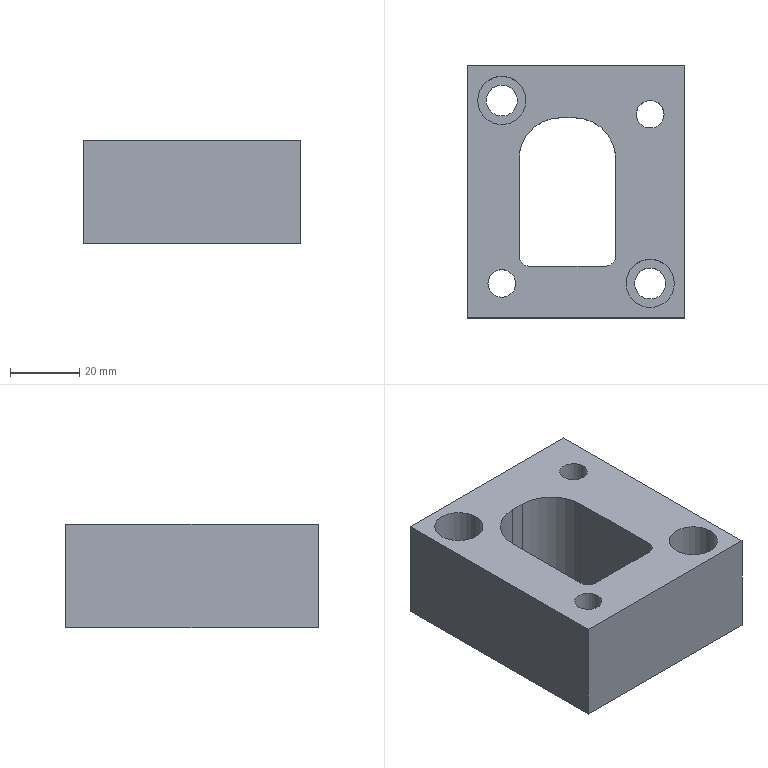Part | STEP file | 1 solid | 22 faces | box 63 x 73 x 30 mm | volume 93374 mm3 | plane 12 | cylinder 10 | commonest cylinder face diameters 6 x2 8 x2 9 x2 14 x2 24 x2
STEP:
#1=CARTESIAN_POINT('',(-173.586,-75.,-2.));
#2=VERTEX_POINT('',#1);
#3=CARTESIAN_POINT('',(-177.586,-75.,-2.));
#4=DIRECTION('',(0.,0.,-1.));
#5=DIRECTION('',(1.,0.,0.));
#6=AXIS2_PLACEMENT_3D('',#3,#4,#5);
#7=CIRCLE('',#6,4.);
#8=EDGE_CURVE('',#2,#2,#7,.T.);
#9=ORIENTED_EDGE('',*,*,#8,.T.);
#10=EDGE_LOOP('',(#9));
#11=FACE_BOUND('',#10,.T.);
#12=CARTESIAN_POINT('',(-216.586,-124.,-2.));
#13=VERTEX_POINT('',#12);
#14=CARTESIAN_POINT('',(-220.586,-124.,-2.));
#15=DIRECTION('',(0.,0.,-1.));
#16=DIRECTION('',(1.,0.,0.));
#17=AXIS2_PLACEMENT_3D('',#14,#15,#16);
#18=CIRCLE('',#17,4.);
#19=EDGE_CURVE('',#13,#13,#18,.T.);
#20=ORIENTED_EDGE('',*,*,#19,.T.);
#21=EDGE_LOOP('',(#20));
#22=FACE_BOUND('',#21,.T.);
#23=CARTESIAN_POINT('',(-227.586,-71.,-2.));
#24=VERTEX_POINT('',#23);
#25=CARTESIAN_POINT('',(-220.586,-71.,-2.));
#26=DIRECTION('',(0.,0.,-1.));
#27=DIRECTION('',(-1.,0.,0.));
#28=AXIS2_PLACEMENT_3D('',#25,#26,#27);
#29=CIRCLE('',#28,7.);
#30=EDGE_CURVE('',#24,#24,#29,.T.);
#31=ORIENTED_EDGE('',*,*,#30,.T.);
#32=EDGE_LOOP('',(#31));
#33=FACE_BOUND('',#32,.T.);
#34=CARTESIAN_POINT('',(-170.586,-124.,-2.));
#35=VERTEX_POINT('',#34);
#36=CARTESIAN_POINT('',(-177.586,-124.,-2.));
#37=DIRECTION('',(0.,0.,-1.));
#38=DIRECTION('',(1.,0.,0.));
#39=AXIS2_PLACEMENT_3D('',#36,#37,#38);
#40=CIRCLE('',#39,7.);
#41=EDGE_CURVE('',#35,#35,#40,.T.);
#42=ORIENTED_EDGE('',*,*,#41,.T.);
#43=EDGE_LOOP('',(#42));
#44=FACE_BOUND('',#43,.T.);
#45=CARTESIAN_POINT('',(-199.586,-76.,-2.));
#46=VERTEX_POINT('',#45);
#47=CARTESIAN_POINT('',(-187.586,-88.,-2.));
#48=VERTEX_POINT('',#47);
#49=CARTESIAN_POINT('',(-199.586,-88.,-2.));
#50=DIRECTION('',(0.,0.,-1.));
#51=DIRECTION('',(1.,0.,0.));
#52=AXIS2_PLACEMENT_3D('',#49,#50,#51);
#53=CIRCLE('',#52,12.);
#54=EDGE_CURVE('',#46,#48,#53,.T.);
#55=ORIENTED_EDGE('',*,*,#54,.T.);
#56=CARTESIAN_POINT('',(-187.586,-116.,-2.));
#57=VERTEX_POINT('',#56);
#58=CARTESIAN_POINT('',(-187.586,-97.5,-2.));
#59=DIRECTION('',(0.,-1.,0.));
#60=VECTOR('',#59,1.);
#61=LINE('',#58,#60);
#62=EDGE_CURVE('',#48,#57,#61,.T.);
#63=ORIENTED_EDGE('',*,*,#62,.T.);
#64=CARTESIAN_POINT('',(-190.586,-119.,-2.));
#65=VERTEX_POINT('',#64);
#66=CARTESIAN_POINT('',(-190.586,-116.,-2.));
#67=DIRECTION('',(0.,0.,-1.));
#68=DIRECTION('',(1.,0.,0.));
#69=AXIS2_PLACEMENT_3D('',#66,#67,#68);
#70=CIRCLE('',#69,3.);
#71=EDGE_CURVE('',#57,#65,#70,.T.);
#72=ORIENTED_EDGE('',*,*,#71,.T.);
#73=CARTESIAN_POINT('',(-212.586,-119.,-2.));
#74=VERTEX_POINT('',#73);
#75=CARTESIAN_POINT('',(-201.586,-119.,-2.));
#76=DIRECTION('',(-1.,0.,0.));
#77=VECTOR('',#76,1.);
#78=LINE('',#75,#77);
#79=EDGE_CURVE('',#65,#74,#78,.T.);
#80=ORIENTED_EDGE('',*,*,#79,.T.);
#81=CARTESIAN_POINT('',(-215.586,-116.,-2.));
#82=VERTEX_POINT('',#81);
#83=CARTESIAN_POINT('',(-212.586,-116.,-2.));
#84=DIRECTION('',(0.,0.,-1.));
#85=DIRECTION('',(1.,0.,0.));
#86=AXIS2_PLACEMENT_3D('',#83,#84,#85);
#87=CIRCLE('',#86,3.);
#88=EDGE_CURVE('',#74,#82,#87,.T.);
#89=ORIENTED_EDGE('',*,*,#88,.T.);
#90=CARTESIAN_POINT('',(-215.586,-88.,-2.));
#91=VERTEX_POINT('',#90);
#92=CARTESIAN_POINT('',(-215.586,-97.5,-2.));
#93=DIRECTION('',(0.,1.,0.));
#94=VECTOR('',#93,1.);
#95=LINE('',#92,#94);
#96=EDGE_CURVE('',#82,#91,#95,.T.);
#97=ORIENTED_EDGE('',*,*,#96,.T.);
#98=CARTESIAN_POINT('',(-203.586,-76.,-2.));
#99=VERTEX_POINT('',#98);
#100=CARTESIAN_POINT('',(-203.586,-88.,-2.));
#101=DIRECTION('',(0.,0.,-1.));
#102=DIRECTION('',(1.,0.,0.));
#103=AXIS2_PLACEMENT_3D('',#100,#101,#102);
#104=CIRCLE('',#103,12.);
#105=EDGE_CURVE('',#91,#99,#104,.T.);
#106=ORIENTED_EDGE('',*,*,#105,.T.);
#107=CARTESIAN_POINT('',(-201.586,-76.,-2.));
#108=DIRECTION('',(1.,0.,0.));
#109=VECTOR('',#108,1.);
#110=LINE('',#107,#109);
#111=EDGE_CURVE('',#99,#46,#110,.T.);
#112=ORIENTED_EDGE('',*,*,#111,.T.);
#113=EDGE_LOOP('',(#55,#63,#72,#80,#89,#97,#106,#112));
#114=FACE_BOUND('',#113,.T.);
#115=CARTESIAN_POINT('',(-167.586,-61.,-2.));
#116=VERTEX_POINT('',#115);
#117=CARTESIAN_POINT('',(-167.586,-134.,-2.));
#118=VERTEX_POINT('',#117);
#119=CARTESIAN_POINT('',(-167.586,-97.5,-2.));
#120=DIRECTION('',(0.,-1.,0.));
#121=VECTOR('',#120,1.);
#122=LINE('',#119,#121);
#123=EDGE_CURVE('',#116,#118,#122,.T.);
#124=ORIENTED_EDGE('',*,*,#123,.F.);
#125=CARTESIAN_POINT('',(-230.586,-61.,-2.));
#126=VERTEX_POINT('',#125);
#127=CARTESIAN_POINT('',(-201.586,-61.,-2.));
#128=DIRECTION('',(1.,0.,0.));
#129=VECTOR('',#128,1.);
#130=LINE('',#127,#129);
#131=EDGE_CURVE('',#126,#116,#130,.T.);
#132=ORIENTED_EDGE('',*,*,#131,.F.);
#133=CARTESIAN_POINT('',(-230.586,-134.,-2.));
#134=VERTEX_POINT('',#133);
#135=CARTESIAN_POINT('',(-230.586,-97.5,-2.));
#136=DIRECTION('',(0.,1.,0.));
#137=VECTOR('',#136,1.);
#138=LINE('',#135,#137);
#139=EDGE_CURVE('',#134,#126,#138,.T.);
#140=ORIENTED_EDGE('',*,*,#139,.F.);
#141=CARTESIAN_POINT('',(-201.586,-134.,-2.));
#142=DIRECTION('',(-1.,0.,0.));
#143=VECTOR('',#142,1.);
#144=LINE('',#141,#143);
#145=EDGE_CURVE('',#118,#134,#144,.T.);
#146=ORIENTED_EDGE('',*,*,#145,.F.);
#147=EDGE_LOOP('',(#124,#132,#140,#146));
#148=FACE_BOUND('',#147,.T.);
#149=CARTESIAN_POINT('',(-201.586,-97.5,-2.));
#150=DIRECTION('',(0.,0.,1.));
#151=DIRECTION('',(1.,0.,0.));
#152=AXIS2_PLACEMENT_3D('',#149,#150,#151);
#153=PLANE('',#152);
#154=ADVANCED_FACE('',(#11,#22,#33,#44,#114,#148),#153,.T.);
#155=CARTESIAN_POINT('',(-167.586,-134.,-32.));
#156=VERTEX_POINT('',#155);
#157=CARTESIAN_POINT('',(-167.586,-134.,-52.));
#158=DIRECTION('',(0.,0.,1.));
#159=VECTOR('',#158,1.);
#160=LINE('',#157,#159);
#161=EDGE_CURVE('',#156,#118,#160,.T.);
#162=ORIENTED_EDGE('',*,*,#161,.T.);
#163=ORIENTED_EDGE('',*,*,#145,.T.);
#164=CARTESIAN_POINT('',(-230.586,-134.,-32.));
#165=VERTEX_POINT('',#164);
#166=CARTESIAN_POINT('',(-230.586,-134.,-52.));
#167=DIRECTION('',(0.,0.,1.));
#168=VECTOR('',#167,1.);
#169=LINE('',#166,#168);
#170=EDGE_CURVE('',#165,#134,#169,.T.);
#171=ORIENTED_EDGE('',*,*,#170,.F.);
#172=CARTESIAN_POINT('',(-201.586,-134.,-32.));
#173=DIRECTION('',(1.,0.,0.));
#174=VECTOR('',#173,1.);
#175=LINE('',#172,#174);
#176=EDGE_CURVE('',#165,#156,#175,.T.);
#177=ORIENTED_EDGE('',*,*,#176,.T.);
#178=EDGE_LOOP('',(#162,#163,#171,#177));
#179=FACE_OUTER_BOUND('',#178,.T.);
#180=CARTESIAN_POINT('',(-201.586,-134.,-52.));
#181=DIRECTION('',(0.,-1.,0.));
#182=DIRECTION('',(0.,0.,-1.));
#183=AXIS2_PLACEMENT_3D('',#180,#181,#182);
#184=PLANE('',#183);
#185=ADVANCED_FACE('',(#179),#184,.T.);
#186=ORIENTED_EDGE('',*,*,#170,.T.);
#187=ORIENTED_EDGE('',*,*,#139,.T.);
#188=CARTESIAN_POINT('',(-230.586,-61.,-32.));
#189=VERTEX_POINT('',#188);
#190=CARTESIAN_POINT('',(-230.586,-61.,-52.));
#191=DIRECTION('',(0.,0.,1.));
#192=VECTOR('',#191,1.);
#193=LINE('',#190,#192);
#194=EDGE_CURVE('',#189,#126,#193,.T.);
#195=ORIENTED_EDGE('',*,*,#194,.F.);
#196=CARTESIAN_POINT('',(-230.586,-97.5,-32.));
#197=DIRECTION('',(0.,-1.,0.));
#198=VECTOR('',#197,1.);
#199=LINE('',#196,#198);
#200=EDGE_CURVE('',#189,#165,#199,.T.);
#201=ORIENTED_EDGE('',*,*,#200,.T.);
#202=EDGE_LOOP('',(#186,#187,#195,#201));
#203=FACE_OUTER_BOUND('',#202,.T.);
#204=CARTESIAN_POINT('',(-230.586,-97.5,-52.));
#205=DIRECTION('',(-1.,0.,0.));
#206=DIRECTION('',(0.,0.,1.));
#207=AXIS2_PLACEMENT_3D('',#204,#205,#206);
#208=PLANE('',#207);
#209=ADVANCED_FACE('',(#203),#208,.T.);
#210=ORIENTED_EDGE('',*,*,#131,.T.);
#211=CARTESIAN_POINT('',(-167.586,-61.,-32.));
#212=VERTEX_POINT('',#211);
#213=CARTESIAN_POINT('',(-167.586,-61.,-52.));
#214=DIRECTION('',(0.,0.,-1.));
#215=VECTOR('',#214,1.);
#216=LINE('',#213,#215);
#217=EDGE_CURVE('',#116,#212,#216,.T.);
#218=ORIENTED_EDGE('',*,*,#217,.T.);
#219=CARTESIAN_POINT('',(-201.586,-61.,-32.));
#220=DIRECTION('',(-1.,0.,0.));
#221=VECTOR('',#220,1.);
#222=LINE('',#219,#221);
#223=EDGE_CURVE('',#212,#189,#222,.T.);
#224=ORIENTED_EDGE('',*,*,#223,.T.);
#225=ORIENTED_EDGE('',*,*,#194,.T.);
#226=EDGE_LOOP('',(#210,#218,#224,#225));
#227=FACE_OUTER_BOUND('',#226,.T.);
#228=CARTESIAN_POINT('',(-201.586,-61.,-52.));
#229=DIRECTION('',(0.,1.,0.));
#230=DIRECTION('',(0.,0.,1.));
#231=AXIS2_PLACEMENT_3D('',#228,#229,#230);
#232=PLANE('',#231);
#233=ADVANCED_FACE('',(#227),#232,.T.);
#234=CARTESIAN_POINT('',(-225.086,-71.,-32.));
#235=VERTEX_POINT('',#234);
#236=CARTESIAN_POINT('',(-220.586,-71.,-32.));
#237=DIRECTION('',(0.,0.,-1.));
#238=DIRECTION('',(-1.,0.,0.));
#239=AXIS2_PLACEMENT_3D('',#236,#237,#238);
#240=CIRCLE('',#239,4.5);
#241=EDGE_CURVE('',#235,#235,#240,.T.);
#242=ORIENTED_EDGE('',*,*,#241,.F.);
#243=EDGE_LOOP('',(#242));
#244=FACE_BOUND('',#243,.T.);
#245=CARTESIAN_POINT('',(-182.086,-124.,-32.));
#246=VERTEX_POINT('',#245);
#247=CARTESIAN_POINT('',(-177.586,-124.,-32.));
#248=DIRECTION('',(0.,0.,-1.));
#249=DIRECTION('',(-1.,0.,0.));
#250=AXIS2_PLACEMENT_3D('',#247,#248,#249);
#251=CIRCLE('',#250,4.5);
#252=EDGE_CURVE('',#246,#246,#251,.T.);
#253=ORIENTED_EDGE('',*,*,#252,.F.);
#254=EDGE_LOOP('',(#253));
#255=FACE_BOUND('',#254,.T.);
#256=CARTESIAN_POINT('',(-190.586,-119.,-32.));
#257=VERTEX_POINT('',#256);
#258=CARTESIAN_POINT('',(-187.586,-116.,-32.));
#259=VERTEX_POINT('',#258);
#260=CARTESIAN_POINT('',(-190.586,-116.,-32.));
#261=DIRECTION('',(0.,0.,1.));
#262=DIRECTION('',(-1.,0.,0.));
#263=AXIS2_PLACEMENT_3D('',#260,#261,#262);
#264=CIRCLE('',#263,3.);
#265=EDGE_CURVE('',#257,#259,#264,.T.);
#266=ORIENTED_EDGE('',*,*,#265,.T.);
#267=CARTESIAN_POINT('',(-187.586,-88.,-32.));
#268=VERTEX_POINT('',#267);
#269=CARTESIAN_POINT('',(-187.586,-97.5,-32.));
#270=DIRECTION('',(0.,1.,0.));
#271=VECTOR('',#270,1.);
#272=LINE('',#269,#271);
#273=EDGE_CURVE('',#259,#268,#272,.T.);
#274=ORIENTED_EDGE('',*,*,#273,.T.);
#275=CARTESIAN_POINT('',(-199.586,-76.,-32.));
#276=VERTEX_POINT('',#275);
#277=CARTESIAN_POINT('',(-199.586,-88.,-32.));
#278=DIRECTION('',(0.,0.,1.));
#279=DIRECTION('',(-1.,0.,0.));
#280=AXIS2_PLACEMENT_3D('',#277,#278,#279);
#281=CIRCLE('',#280,12.);
#282=EDGE_CURVE('',#268,#276,#281,.T.);
#283=ORIENTED_EDGE('',*,*,#282,.T.);
#284=CARTESIAN_POINT('',(-203.586,-76.,-32.));
#285=VERTEX_POINT('',#284);
#286=CARTESIAN_POINT('',(-201.586,-76.,-32.));
#287=DIRECTION('',(-1.,0.,0.));
#288=VECTOR('',#287,1.);
#289=LINE('',#286,#288);
#290=EDGE_CURVE('',#276,#285,#289,.T.);
#291=ORIENTED_EDGE('',*,*,#290,.T.);
#292=CARTESIAN_POINT('',(-215.586,-88.,-32.));
#293=VERTEX_POINT('',#292);
#294=CARTESIAN_POINT('',(-203.586,-88.,-32.));
#295=DIRECTION('',(0.,0.,1.));
#296=DIRECTION('',(-1.,0.,0.));
#297=AXIS2_PLACEMENT_3D('',#294,#295,#296);
#298=CIRCLE('',#297,12.);
#299=EDGE_CURVE('',#285,#293,#298,.T.);
#300=ORIENTED_EDGE('',*,*,#299,.T.);
#301=CARTESIAN_POINT('',(-215.586,-116.,-32.));
#302=VERTEX_POINT('',#301);
#303=CARTESIAN_POINT('',(-215.586,-97.5,-32.));
#304=DIRECTION('',(0.,-1.,0.));
#305=VECTOR('',#304,1.);
#306=LINE('',#303,#305);
#307=EDGE_CURVE('',#293,#302,#306,.T.);
#308=ORIENTED_EDGE('',*,*,#307,.T.);
#309=CARTESIAN_POINT('',(-212.586,-119.,-32.));
#310=VERTEX_POINT('',#309);
#311=CARTESIAN_POINT('',(-212.586,-116.,-32.));
#312=DIRECTION('',(0.,0.,1.));
#313=DIRECTION('',(-1.,0.,0.));
#314=AXIS2_PLACEMENT_3D('',#311,#312,#313);
#315=CIRCLE('',#314,3.);
#316=EDGE_CURVE('',#302,#310,#315,.T.);
#317=ORIENTED_EDGE('',*,*,#316,.T.);
#318=CARTESIAN_POINT('',(-201.586,-119.,-32.));
#319=DIRECTION('',(1.,0.,0.));
#320=VECTOR('',#319,1.);
#321=LINE('',#318,#320);
#322=EDGE_CURVE('',#310,#257,#321,.T.);
#323=ORIENTED_EDGE('',*,*,#322,.T.);
#324=EDGE_LOOP('',(#266,#274,#283,#291,#300,#308,#317,#323));
#325=FACE_BOUND('',#324,.T.);
#326=ORIENTED_EDGE('',*,*,#223,.F.);
#327=CARTESIAN_POINT('',(-167.586,-97.5,-32.));
#328=DIRECTION('',(0.,1.,0.));
#329=VECTOR('',#328,1.);
#330=LINE('',#327,#329);
#331=EDGE_CURVE('',#156,#212,#330,.T.);
#332=ORIENTED_EDGE('',*,*,#331,.F.);
#333=ORIENTED_EDGE('',*,*,#176,.F.);
#334=ORIENTED_EDGE('',*,*,#200,.F.);
#335=EDGE_LOOP('',(#326,#332,#333,#334));
#336=FACE_BOUND('',#335,.T.);
#337=CARTESIAN_POINT('',(-216.586,-124.,-32.));
#338=VERTEX_POINT('',#337);
#339=CARTESIAN_POINT('',(-220.586,-124.,-32.));
#340=DIRECTION('',(0.,0.,-1.));
#341=DIRECTION('',(1.,0.,0.));
#342=AXIS2_PLACEMENT_3D('',#339,#340,#341);
#343=CIRCLE('',#342,4.);
#344=EDGE_CURVE('',#338,#338,#343,.T.);
#345=ORIENTED_EDGE('',*,*,#344,.F.);
#346=EDGE_LOOP('',(#345));
#347=FACE_BOUND('',#346,.T.);
#348=CARTESIAN_POINT('',(-173.586,-75.,-32.));
#349=VERTEX_POINT('',#348);
#350=CARTESIAN_POINT('',(-177.586,-75.,-32.));
#351=DIRECTION('',(0.,0.,-1.));
#352=DIRECTION('',(1.,0.,0.));
#353=AXIS2_PLACEMENT_3D('',#350,#351,#352);
#354=CIRCLE('',#353,4.);
#355=EDGE_CURVE('',#349,#349,#354,.T.);
#356=ORIENTED_EDGE('',*,*,#355,.F.);
#357=EDGE_LOOP('',(#356));
#358=FACE_BOUND('',#357,.T.);
#359=CARTESIAN_POINT('',(-201.586,-97.5,-32.));
#360=DIRECTION('',(0.,0.,-1.));
#361=DIRECTION('',(-1.,0.,0.));
#362=AXIS2_PLACEMENT_3D('',#359,#360,#361);
#363=PLANE('',#362);
#364=ADVANCED_FACE('',(#244,#255,#325,#336,#347,#358),#363,.T.);
#365=ORIENTED_EDGE('',*,*,#331,.T.);
#366=ORIENTED_EDGE('',*,*,#217,.F.);
#367=ORIENTED_EDGE('',*,*,#123,.T.);
#368=ORIENTED_EDGE('',*,*,#161,.F.);
#369=EDGE_LOOP('',(#365,#366,#367,#368));
#370=FACE_OUTER_BOUND('',#369,.T.);
#371=CARTESIAN_POINT('',(-167.586,-97.5,-52.));
#372=DIRECTION('',(1.,0.,0.));
#373=DIRECTION('',(0.,0.,-1.));
#374=AXIS2_PLACEMENT_3D('',#371,#372,#373);
#375=PLANE('',#374);
#376=ADVANCED_FACE('',(#370),#375,.T.);
#377=CARTESIAN_POINT('',(-187.586,-88.,113.));
#378=DIRECTION('',(0.,0.,1.));
#379=VECTOR('',#378,1.);
#380=LINE('',#377,#379);
#381=EDGE_CURVE('',#268,#48,#380,.T.);
#382=ORIENTED_EDGE('',*,*,#381,.F.);
#383=ORIENTED_EDGE('',*,*,#273,.F.);
#384=CARTESIAN_POINT('',(-187.586,-116.,113.));
#385=DIRECTION('',(0.,0.,1.));
#386=VECTOR('',#385,1.);
#387=LINE('',#384,#386);
#388=EDGE_CURVE('',#259,#57,#387,.T.);
#389=ORIENTED_EDGE('',*,*,#388,.T.);
#390=ORIENTED_EDGE('',*,*,#62,.F.);
#391=EDGE_LOOP('',(#382,#383,#389,#390));
#392=FACE_OUTER_BOUND('',#391,.T.);
#393=CARTESIAN_POINT('',(-187.586,-116.,113.));
#394=DIRECTION('',(-1.,0.,0.));
#395=DIRECTION('',(0.,0.,1.));
#396=AXIS2_PLACEMENT_3D('',#393,#394,#395);
#397=PLANE('',#396);
#398=ADVANCED_FACE('',(#392),#397,.T.);
#399=CARTESIAN_POINT('',(-199.586,-76.,113.));
#400=DIRECTION('',(0.,0.,1.));
#401=VECTOR('',#400,1.);
#402=LINE('',#399,#401);
#403=EDGE_CURVE('',#276,#46,#402,.T.);
#404=ORIENTED_EDGE('',*,*,#403,.F.);
#405=ORIENTED_EDGE('',*,*,#282,.F.);
#406=ORIENTED_EDGE('',*,*,#381,.T.);
#407=ORIENTED_EDGE('',*,*,#54,.F.);
#408=EDGE_LOOP('',(#404,#405,#406,#407));
#409=FACE_OUTER_BOUND('',#408,.T.);
#410=CARTESIAN_POINT('',(-199.586,-88.,113.));
#411=DIRECTION('',(0.,0.,-1.));
#412=DIRECTION('',(-1.,0.,0.));
#413=AXIS2_PLACEMENT_3D('',#410,#411,#412);
#414=CYLINDRICAL_SURFACE('',#413,12.);
#415=ADVANCED_FACE('',(#409),#414,.F.);
#416=CARTESIAN_POINT('',(-203.586,-76.,113.));
#417=DIRECTION('',(0.,0.,1.));
#418=VECTOR('',#417,1.);
#419=LINE('',#416,#418);
#420=EDGE_CURVE('',#285,#99,#419,.T.);
#421=ORIENTED_EDGE('',*,*,#420,.F.);
#422=ORIENTED_EDGE('',*,*,#290,.F.);
#423=ORIENTED_EDGE('',*,*,#403,.T.);
#424=ORIENTED_EDGE('',*,*,#111,.F.);
#425=EDGE_LOOP('',(#421,#422,#423,#424));
#426=FACE_OUTER_BOUND('',#425,.T.);
#427=CARTESIAN_POINT('',(-199.586,-76.,113.));
#428=DIRECTION('',(0.,-1.,0.));
#429=DIRECTION('',(0.,0.,-1.));
#430=AXIS2_PLACEMENT_3D('',#427,#428,#429);
#431=PLANE('',#430);
#432=ADVANCED_FACE('',(#426),#431,.T.);
#433=CARTESIAN_POINT('',(-215.586,-88.,113.));
#434=DIRECTION('',(0.,0.,1.));
#435=VECTOR('',#434,1.);
#436=LINE('',#433,#435);
#437=EDGE_CURVE('',#293,#91,#436,.T.);
#438=ORIENTED_EDGE('',*,*,#437,.F.);
#439=ORIENTED_EDGE('',*,*,#299,.F.);
#440=ORIENTED_EDGE('',*,*,#420,.T.);
#441=ORIENTED_EDGE('',*,*,#105,.F.);
#442=EDGE_LOOP('',(#438,#439,#440,#441));
#443=FACE_OUTER_BOUND('',#442,.T.);
#444=CARTESIAN_POINT('',(-203.586,-88.,113.));
#445=DIRECTION('',(0.,0.,-1.));
#446=DIRECTION('',(-1.,0.,0.));
#447=AXIS2_PLACEMENT_3D('',#444,#445,#446);
#448=CYLINDRICAL_SURFACE('',#447,12.);
#449=ADVANCED_FACE('',(#443),#448,.F.);
#450=CARTESIAN_POINT('',(-215.586,-116.,113.));
#451=DIRECTION('',(0.,0.,1.));
#452=VECTOR('',#451,1.);
#453=LINE('',#450,#452);
#454=EDGE_CURVE('',#302,#82,#453,.T.);
#455=ORIENTED_EDGE('',*,*,#454,.F.);
#456=ORIENTED_EDGE('',*,*,#307,.F.);
#457=ORIENTED_EDGE('',*,*,#437,.T.);
#458=ORIENTED_EDGE('',*,*,#96,.F.);
#459=EDGE_LOOP('',(#455,#456,#457,#458));
#460=FACE_OUTER_BOUND('',#459,.T.);
#461=CARTESIAN_POINT('',(-215.586,-88.,113.));
#462=DIRECTION('',(1.,0.,0.));
#463=DIRECTION('',(0.,0.,-1.));
#464=AXIS2_PLACEMENT_3D('',#461,#462,#463);
#465=PLANE('',#464);
#466=ADVANCED_FACE('',(#460),#465,.T.);
#467=CARTESIAN_POINT('',(-212.586,-119.,113.));
#468=DIRECTION('',(0.,0.,1.));
#469=VECTOR('',#468,1.);
#470=LINE('',#467,#469);
#471=EDGE_CURVE('',#310,#74,#470,.T.);
#472=ORIENTED_EDGE('',*,*,#471,.F.);
#473=ORIENTED_EDGE('',*,*,#316,.F.);
#474=ORIENTED_EDGE('',*,*,#454,.T.);
#475=ORIENTED_EDGE('',*,*,#88,.F.);
#476=EDGE_LOOP('',(#472,#473,#474,#475));
#477=FACE_OUTER_BOUND('',#476,.T.);
#478=CARTESIAN_POINT('',(-212.586,-116.,113.));
#479=DIRECTION('',(0.,0.,-1.));
#480=DIRECTION('',(-1.,0.,0.));
#481=AXIS2_PLACEMENT_3D('',#478,#479,#480);
#482=CYLINDRICAL_SURFACE('',#481,3.);
#483=ADVANCED_FACE('',(#477),#482,.F.);
#484=CARTESIAN_POINT('',(-190.586,-119.,113.));
#485=DIRECTION('',(0.,0.,1.));
#486=VECTOR('',#485,1.);
#487=LINE('',#484,#486);
#488=EDGE_CURVE('',#257,#65,#487,.T.);
#489=ORIENTED_EDGE('',*,*,#488,.F.);
#490=ORIENTED_EDGE('',*,*,#322,.F.);
#491=ORIENTED_EDGE('',*,*,#471,.T.);
#492=ORIENTED_EDGE('',*,*,#79,.F.);
#493=EDGE_LOOP('',(#489,#490,#491,#492));
#494=FACE_OUTER_BOUND('',#493,.T.);
#495=CARTESIAN_POINT('',(-212.586,-119.,113.));
#496=DIRECTION('',(0.,1.,0.));
#497=DIRECTION('',(0.,0.,1.));
#498=AXIS2_PLACEMENT_3D('',#495,#496,#497);
#499=PLANE('',#498);
#500=ADVANCED_FACE('',(#494),#499,.T.);
#501=ORIENTED_EDGE('',*,*,#388,.F.);
#502=ORIENTED_EDGE('',*,*,#265,.F.);
#503=ORIENTED_EDGE('',*,*,#488,.T.);
#504=ORIENTED_EDGE('',*,*,#71,.F.);
#505=EDGE_LOOP('',(#501,#502,#503,#504));
#506=FACE_OUTER_BOUND('',#505,.T.);
#507=CARTESIAN_POINT('',(-190.586,-116.,113.));
#508=DIRECTION('',(0.,0.,-1.));
#509=DIRECTION('',(-1.,0.,0.));
#510=AXIS2_PLACEMENT_3D('',#507,#508,#509);
#511=CYLINDRICAL_SURFACE('',#510,3.);
#512=ADVANCED_FACE('',(#506),#511,.F.);
#513=ORIENTED_EDGE('',*,*,#252,.T.);
#514=EDGE_LOOP('',(#513));
#515=FACE_BOUND('',#514,.T.);
#516=CARTESIAN_POINT('',(-182.086,-124.,-22.));
#517=VERTEX_POINT('',#516);
#518=CARTESIAN_POINT('',(-177.586,-124.,-22.));
#519=DIRECTION('',(0.,0.,-1.));
#520=DIRECTION('',(-1.,0.,0.));
#521=AXIS2_PLACEMENT_3D('',#518,#519,#520);
#522=CIRCLE('',#521,4.5);
#523=EDGE_CURVE('',#517,#517,#522,.T.);
#524=ORIENTED_EDGE('',*,*,#523,.F.);
#525=EDGE_LOOP('',(#524));
#526=FACE_BOUND('',#525,.T.);
#527=CARTESIAN_POINT('',(-177.586,-124.,-47.));
#528=DIRECTION('',(0.,0.,1.));
#529=DIRECTION('',(1.,0.,0.));
#530=AXIS2_PLACEMENT_3D('',#527,#528,#529);
#531=CYLINDRICAL_SURFACE('',#530,4.5);
#532=ADVANCED_FACE('',(#515,#526),#531,.F.);
#533=ORIENTED_EDGE('',*,*,#523,.T.);
#534=EDGE_LOOP('',(#533));
#535=FACE_BOUND('',#534,.T.);
#536=CARTESIAN_POINT('',(-170.586,-124.,-22.));
#537=VERTEX_POINT('',#536);
#538=CARTESIAN_POINT('',(-177.586,-124.,-22.));
#539=DIRECTION('',(0.,0.,-1.));
#540=DIRECTION('',(1.,0.,0.));
#541=AXIS2_PLACEMENT_3D('',#538,#539,#540);
#542=CIRCLE('',#541,7.);
#543=EDGE_CURVE('',#537,#537,#542,.T.);
#544=ORIENTED_EDGE('',*,*,#543,.F.);
#545=EDGE_LOOP('',(#544));
#546=FACE_BOUND('',#545,.T.);
#547=CARTESIAN_POINT('',(-177.586,-124.,-22.));
#548=DIRECTION('',(0.,0.,-1.));
#549=DIRECTION('',(-1.,0.,0.));
#550=AXIS2_PLACEMENT_3D('',#547,#548,#549);
#551=PLANE('',#550);
#552=ADVANCED_FACE('',(#535,#546),#551,.F.);
#553=ORIENTED_EDGE('',*,*,#41,.F.);
#554=EDGE_LOOP('',(#553));
#555=FACE_BOUND('',#554,.T.);
#556=ORIENTED_EDGE('',*,*,#543,.T.);
#557=EDGE_LOOP('',(#556));
#558=FACE_BOUND('',#557,.T.);
#559=CARTESIAN_POINT('',(-177.586,-124.,-22.));
#560=DIRECTION('',(0.,0.,1.));
#561=DIRECTION('',(1.,0.,0.));
#562=AXIS2_PLACEMENT_3D('',#559,#560,#561);
#563=CYLINDRICAL_SURFACE('',#562,7.);
#564=ADVANCED_FACE('',(#555,#558),#563,.F.);
#565=ORIENTED_EDGE('',*,*,#241,.T.);
#566=EDGE_LOOP('',(#565));
#567=FACE_BOUND('',#566,.T.);
#568=CARTESIAN_POINT('',(-216.086,-71.,-22.));
#569=VERTEX_POINT('',#568);
#570=CARTESIAN_POINT('',(-220.586,-71.,-22.));
#571=DIRECTION('',(0.,0.,-1.));
#572=DIRECTION('',(1.,0.,0.));
#573=AXIS2_PLACEMENT_3D('',#570,#571,#572);
#574=CIRCLE('',#573,4.5);
#575=EDGE_CURVE('',#569,#569,#574,.T.);
#576=ORIENTED_EDGE('',*,*,#575,.F.);
#577=EDGE_LOOP('',(#576));
#578=FACE_BOUND('',#577,.T.);
#579=CARTESIAN_POINT('',(-220.586,-71.,-47.));
#580=DIRECTION('',(0.,0.,1.));
#581=DIRECTION('',(-1.,0.,0.));
#582=AXIS2_PLACEMENT_3D('',#579,#580,#581);
#583=CYLINDRICAL_SURFACE('',#582,4.5);
#584=ADVANCED_FACE('',(#567,#578),#583,.F.);
#585=ORIENTED_EDGE('',*,*,#575,.T.);
#586=EDGE_LOOP('',(#585));
#587=FACE_BOUND('',#586,.T.);
#588=CARTESIAN_POINT('',(-227.586,-71.,-22.));
#589=VERTEX_POINT('',#588);
#590=CARTESIAN_POINT('',(-220.586,-71.,-22.));
#591=DIRECTION('',(0.,0.,-1.));
#592=DIRECTION('',(-1.,0.,0.));
#593=AXIS2_PLACEMENT_3D('',#590,#591,#592);
#594=CIRCLE('',#593,7.);
#595=EDGE_CURVE('',#589,#589,#594,.T.);
#596=ORIENTED_EDGE('',*,*,#595,.F.);
#597=EDGE_LOOP('',(#596));
#598=FACE_BOUND('',#597,.T.);
#599=CARTESIAN_POINT('',(-220.586,-71.,-22.));
#600=DIRECTION('',(0.,0.,-1.));
#601=DIRECTION('',(1.,0.,0.));
#602=AXIS2_PLACEMENT_3D('',#599,#600,#601);
#603=PLANE('',#602);
#604=ADVANCED_FACE('',(#587,#598),#603,.F.);
#605=ORIENTED_EDGE('',*,*,#30,.F.);
#606=EDGE_LOOP('',(#605));
#607=FACE_BOUND('',#606,.T.);
#608=ORIENTED_EDGE('',*,*,#595,.T.);
#609=EDGE_LOOP('',(#608));
#610=FACE_BOUND('',#609,.T.);
#611=CARTESIAN_POINT('',(-220.586,-71.,-22.));
#612=DIRECTION('',(0.,0.,1.));
#613=DIRECTION('',(-1.,0.,0.));
#614=AXIS2_PLACEMENT_3D('',#611,#612,#613);
#615=CYLINDRICAL_SURFACE('',#614,7.);
#616=ADVANCED_FACE('',(#607,#610),#615,.F.);
#617=ORIENTED_EDGE('',*,*,#344,.T.);
#618=EDGE_LOOP('',(#617));
#619=FACE_BOUND('',#618,.T.);
#620=ORIENTED_EDGE('',*,*,#19,.F.);
#621=EDGE_LOOP('',(#620));
#622=FACE_BOUND('',#621,.T.);
#623=CARTESIAN_POINT('',(-220.586,-124.,-47.));
#624=DIRECTION('',(0.,0.,1.));
#625=DIRECTION('',(1.,0.,0.));
#626=AXIS2_PLACEMENT_3D('',#623,#624,#625);
#627=CYLINDRICAL_SURFACE('',#626,4.);
#628=ADVANCED_FACE('',(#619,#622),#627,.F.);
#629=ORIENTED_EDGE('',*,*,#355,.T.);
#630=EDGE_LOOP('',(#629));
#631=FACE_BOUND('',#630,.T.);
#632=ORIENTED_EDGE('',*,*,#8,.F.);
#633=EDGE_LOOP('',(#632));
#634=FACE_BOUND('',#633,.T.);
#635=CARTESIAN_POINT('',(-177.586,-75.,-47.));
#636=DIRECTION('',(0.,0.,1.));
#637=DIRECTION('',(1.,0.,0.));
#638=AXIS2_PLACEMENT_3D('',#635,#636,#637);
#639=CYLINDRICAL_SURFACE('',#638,4.);
#640=ADVANCED_FACE('',(#631,#634),#639,.F.);
#641=CLOSED_SHELL('',(#154,#185,#209,#233,#364,#376,#398,#415,#432,#449,#466,#483,#500,#512,#532,#552,#564,#584,#604,#616,#628,#640));
#642=MANIFOLD_SOLID_BREP('',#641);
#643=(LENGTH_UNIT()NAMED_UNIT(*)SI_UNIT(.MILLI.,.METRE.));
#644=UNCERTAINTY_MEASURE_WITH_UNIT(LENGTH_MEASURE(0.00002),#643,'','');
#645=(NAMED_UNIT(*)PLANE_ANGLE_UNIT()SI_UNIT($,.RADIAN.));
#646=PLANE_ANGLE_MEASURE_WITH_UNIT(PLANE_ANGLE_MEASURE(0.01745),#645);
#647=DIMENSIONAL_EXPONENTS(0.,0.,0.,0.,0.,0.,0.);
#648=(CONVERSION_BASED_UNIT('DEGREE',#646)NAMED_UNIT(#647)PLANE_ANGLE_UNIT());
#649=(NAMED_UNIT(*)SI_UNIT($,.STERADIAN.)SOLID_ANGLE_UNIT());
#650=(GEOMETRIC_REPRESENTATION_CONTEXT(3)GLOBAL_UNCERTAINTY_ASSIGNED_CONTEXT((#644))GLOBAL_UNIT_ASSIGNED_CONTEXT((#643,#648,#649))REPRESENTATION_CONTEXT('',''));
#651=ADVANCED_BREP_SHAPE_REPRESENTATION('',(#642),#650);